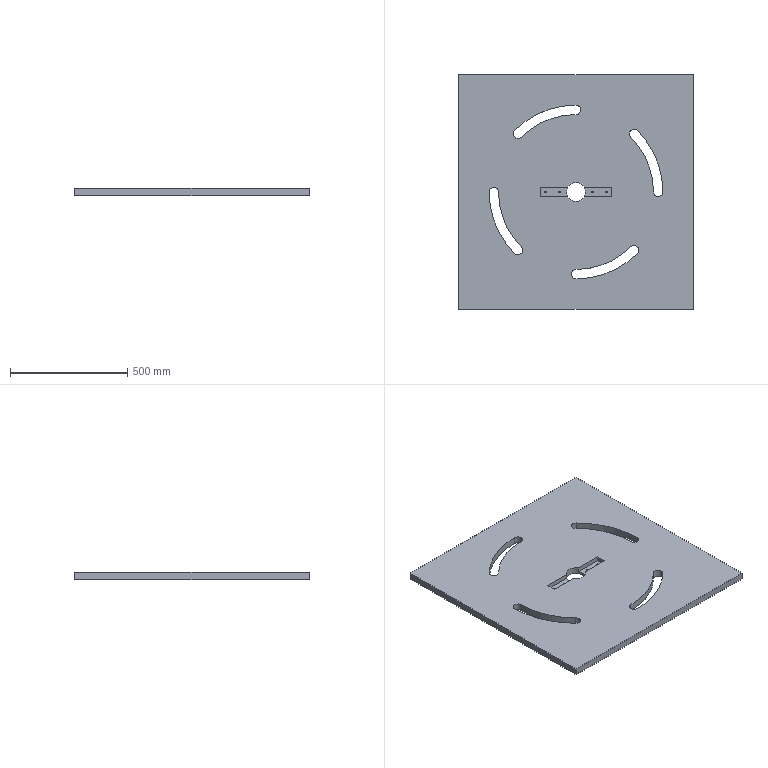Part | SolidWorks | features ICE 3, Extrusion 1, HoleWzd 1 | 1 solid | 43 faces | box 1000 x 1000 x 30 mm | volume 28197892 mm3 | cylinder 29 | plane 14 | commonest cylinder face diameters 40 x11 8.5 x8 660 x4 740 x4 80 x2
STEP:
#1=CARTESIAN_POINT('',(-134.25,0.,0.));
#2=VERTEX_POINT('',#1);
#3=CARTESIAN_POINT('',(-125.75,0.,0.));
#4=VERTEX_POINT('',#3);
#5=CARTESIAN_POINT('',(-130.,0.,0.));
#6=DIRECTION('',(0.,0.,1.));
#7=DIRECTION('',(1.,0.,0.));
#8=AXIS2_PLACEMENT_3D('',#5,#6,#7);
#9=CIRCLE('',#8,4.25);
#10=EDGE_CURVE('',#2,#4,#9,.T.);
#11=ORIENTED_EDGE('',*,*,#10,.F.);
#12=CARTESIAN_POINT('',(-134.25,0.,10.));
#13=VERTEX_POINT('',#12);
#14=CARTESIAN_POINT('',(-134.25,0.,10.));
#15=DIRECTION('',(0.,0.,1.));
#16=VECTOR('',#15,1000.);
#17=LINE('',#14,#16);
#18=EDGE_CURVE('',#2,#13,#17,.T.);
#19=ORIENTED_EDGE('',*,*,#18,.T.);
#20=CARTESIAN_POINT('',(-125.75,0.,10.));
#21=VERTEX_POINT('',#20);
#22=CARTESIAN_POINT('',(-130.,0.,10.));
#23=DIRECTION('',(0.,0.,1.));
#24=DIRECTION('',(1.,0.,0.));
#25=AXIS2_PLACEMENT_3D('',#22,#23,#24);
#26=CIRCLE('',#25,4.25);
#27=EDGE_CURVE('',#13,#21,#26,.T.);
#28=ORIENTED_EDGE('',*,*,#27,.T.);
#29=CARTESIAN_POINT('',(-125.75,0.,10.));
#30=DIRECTION('',(0.,0.,1.));
#31=VECTOR('',#30,1000.);
#32=LINE('',#29,#31);
#33=EDGE_CURVE('',#4,#21,#32,.T.);
#34=ORIENTED_EDGE('',*,*,#33,.F.);
#35=EDGE_LOOP('',(#11,#19,#28,#34));
#36=FACE_OUTER_BOUND('',#35,.T.);
#37=CARTESIAN_POINT('',(-130.,0.,10.));
#38=DIRECTION('',(0.,0.,1.));
#39=DIRECTION('',(1.,0.,0.));
#40=AXIS2_PLACEMENT_3D('',#37,#38,#39);
#41=CYLINDRICAL_SURFACE('',#40,4.25);
#42=ADVANCED_FACE('',(#36),#41,.F.);
#43=CARTESIAN_POINT('',(-74.25,0.,0.));
#44=VERTEX_POINT('',#43);
#45=CARTESIAN_POINT('',(-65.75,0.,0.));
#46=VERTEX_POINT('',#45);
#47=CARTESIAN_POINT('',(-70.,0.,0.));
#48=DIRECTION('',(0.,0.,1.));
#49=DIRECTION('',(1.,0.,0.));
#50=AXIS2_PLACEMENT_3D('',#47,#48,#49);
#51=CIRCLE('',#50,4.25);
#52=EDGE_CURVE('',#44,#46,#51,.T.);
#53=ORIENTED_EDGE('',*,*,#52,.F.);
#54=CARTESIAN_POINT('',(-74.25,0.,10.));
#55=VERTEX_POINT('',#54);
#56=CARTESIAN_POINT('',(-74.25,0.,10.));
#57=DIRECTION('',(0.,0.,1.));
#58=VECTOR('',#57,1000.);
#59=LINE('',#56,#58);
#60=EDGE_CURVE('',#44,#55,#59,.T.);
#61=ORIENTED_EDGE('',*,*,#60,.T.);
#62=CARTESIAN_POINT('',(-65.75,0.,10.));
#63=VERTEX_POINT('',#62);
#64=CARTESIAN_POINT('',(-70.,0.,10.));
#65=DIRECTION('',(0.,0.,1.));
#66=DIRECTION('',(1.,0.,0.));
#67=AXIS2_PLACEMENT_3D('',#64,#65,#66);
#68=CIRCLE('',#67,4.25);
#69=EDGE_CURVE('',#55,#63,#68,.T.);
#70=ORIENTED_EDGE('',*,*,#69,.T.);
#71=CARTESIAN_POINT('',(-65.75,0.,10.));
#72=DIRECTION('',(0.,0.,1.));
#73=VECTOR('',#72,1000.);
#74=LINE('',#71,#73);
#75=EDGE_CURVE('',#46,#63,#74,.T.);
#76=ORIENTED_EDGE('',*,*,#75,.F.);
#77=EDGE_LOOP('',(#53,#61,#70,#76));
#78=FACE_OUTER_BOUND('',#77,.T.);
#79=CARTESIAN_POINT('',(-70.,0.,10.));
#80=DIRECTION('',(0.,0.,1.));
#81=DIRECTION('',(1.,0.,0.));
#82=AXIS2_PLACEMENT_3D('',#79,#80,#81);
#83=CYLINDRICAL_SURFACE('',#82,4.25);
#84=ADVANCED_FACE('',(#78),#83,.F.);
#85=CARTESIAN_POINT('',(65.75,0.,0.));
#86=VERTEX_POINT('',#85);
#87=CARTESIAN_POINT('',(74.25,0.,0.));
#88=VERTEX_POINT('',#87);
#89=CARTESIAN_POINT('',(70.,0.,0.));
#90=DIRECTION('',(0.,0.,1.));
#91=DIRECTION('',(1.,0.,0.));
#92=AXIS2_PLACEMENT_3D('',#89,#90,#91);
#93=CIRCLE('',#92,4.25);
#94=EDGE_CURVE('',#86,#88,#93,.T.);
#95=ORIENTED_EDGE('',*,*,#94,.F.);
#96=CARTESIAN_POINT('',(65.75,0.,10.));
#97=VERTEX_POINT('',#96);
#98=CARTESIAN_POINT('',(65.75,0.,10.));
#99=DIRECTION('',(0.,0.,1.));
#100=VECTOR('',#99,1000.);
#101=LINE('',#98,#100);
#102=EDGE_CURVE('',#86,#97,#101,.T.);
#103=ORIENTED_EDGE('',*,*,#102,.T.);
#104=CARTESIAN_POINT('',(74.25,0.,10.));
#105=VERTEX_POINT('',#104);
#106=CARTESIAN_POINT('',(70.,0.,10.));
#107=DIRECTION('',(0.,0.,1.));
#108=DIRECTION('',(1.,0.,0.));
#109=AXIS2_PLACEMENT_3D('',#106,#107,#108);
#110=CIRCLE('',#109,4.25);
#111=EDGE_CURVE('',#97,#105,#110,.T.);
#112=ORIENTED_EDGE('',*,*,#111,.T.);
#113=CARTESIAN_POINT('',(74.25,0.,10.));
#114=DIRECTION('',(0.,0.,1.));
#115=VECTOR('',#114,1000.);
#116=LINE('',#113,#115);
#117=EDGE_CURVE('',#88,#105,#116,.T.);
#118=ORIENTED_EDGE('',*,*,#117,.F.);
#119=EDGE_LOOP('',(#95,#103,#112,#118));
#120=FACE_OUTER_BOUND('',#119,.T.);
#121=CARTESIAN_POINT('',(70.,0.,10.));
#122=DIRECTION('',(0.,0.,1.));
#123=DIRECTION('',(1.,0.,0.));
#124=AXIS2_PLACEMENT_3D('',#121,#122,#123);
#125=CYLINDRICAL_SURFACE('',#124,4.25);
#126=ADVANCED_FACE('',(#120),#125,.F.);
#127=CARTESIAN_POINT('',(125.75,0.,0.));
#128=VERTEX_POINT('',#127);
#129=CARTESIAN_POINT('',(134.25,0.,0.));
#130=VERTEX_POINT('',#129);
#131=CARTESIAN_POINT('',(130.,0.,0.));
#132=DIRECTION('',(0.,0.,1.));
#133=DIRECTION('',(1.,0.,0.));
#134=AXIS2_PLACEMENT_3D('',#131,#132,#133);
#135=CIRCLE('',#134,4.25);
#136=EDGE_CURVE('',#128,#130,#135,.T.);
#137=ORIENTED_EDGE('',*,*,#136,.F.);
#138=CARTESIAN_POINT('',(125.75,0.,10.));
#139=VERTEX_POINT('',#138);
#140=CARTESIAN_POINT('',(125.75,0.,10.));
#141=DIRECTION('',(0.,0.,1.));
#142=VECTOR('',#141,1000.);
#143=LINE('',#140,#142);
#144=EDGE_CURVE('',#128,#139,#143,.T.);
#145=ORIENTED_EDGE('',*,*,#144,.T.);
#146=CARTESIAN_POINT('',(134.25,0.,10.));
#147=VERTEX_POINT('',#146);
#148=CARTESIAN_POINT('',(130.,0.,10.));
#149=DIRECTION('',(0.,0.,1.));
#150=DIRECTION('',(1.,0.,0.));
#151=AXIS2_PLACEMENT_3D('',#148,#149,#150);
#152=CIRCLE('',#151,4.25);
#153=EDGE_CURVE('',#139,#147,#152,.T.);
#154=ORIENTED_EDGE('',*,*,#153,.T.);
#155=CARTESIAN_POINT('',(134.25,0.,10.));
#156=DIRECTION('',(0.,0.,1.));
#157=VECTOR('',#156,1000.);
#158=LINE('',#155,#157);
#159=EDGE_CURVE('',#130,#147,#158,.T.);
#160=ORIENTED_EDGE('',*,*,#159,.F.);
#161=EDGE_LOOP('',(#137,#145,#154,#160));
#162=FACE_OUTER_BOUND('',#161,.T.);
#163=CARTESIAN_POINT('',(130.,0.,10.));
#164=DIRECTION('',(0.,0.,1.));
#165=DIRECTION('',(1.,0.,0.));
#166=AXIS2_PLACEMENT_3D('',#163,#164,#165);
#167=CYLINDRICAL_SURFACE('',#166,4.25);
#168=ADVANCED_FACE('',(#162),#167,.F.);
#169=CARTESIAN_POINT('',(-40.,0.,0.));
#170=VERTEX_POINT('',#169);
#171=CARTESIAN_POINT('',(40.,0.,0.));
#172=VERTEX_POINT('',#171);
#173=CARTESIAN_POINT('',(0.,0.,0.));
#174=DIRECTION('',(0.,0.,1.));
#175=DIRECTION('',(1.,0.,0.));
#176=AXIS2_PLACEMENT_3D('',#173,#174,#175);
#177=CIRCLE('',#176,40.);
#178=EDGE_CURVE('',#170,#172,#177,.T.);
#179=ORIENTED_EDGE('',*,*,#178,.F.);
#180=CARTESIAN_POINT('',(-40.,0.,10.));
#181=VERTEX_POINT('',#180);
#182=CARTESIAN_POINT('',(-40.,0.,0.));
#183=DIRECTION('',(0.,0.,1.));
#184=VECTOR('',#183,1000.);
#185=LINE('',#182,#184);
#186=EDGE_CURVE('',#170,#181,#185,.T.);
#187=ORIENTED_EDGE('',*,*,#186,.T.);
#188=CARTESIAN_POINT('',(-34.641,-20.,10.));
#189=VERTEX_POINT('',#188);
#190=CARTESIAN_POINT('',(0.,0.,10.));
#191=DIRECTION('',(0.,0.,1.));
#192=DIRECTION('',(-1.,0.,0.));
#193=AXIS2_PLACEMENT_3D('',#190,#191,#192);
#194=CIRCLE('',#193,40.);
#195=EDGE_CURVE('',#181,#189,#194,.T.);
#196=ORIENTED_EDGE('',*,*,#195,.T.);
#197=CARTESIAN_POINT('',(-34.641,-20.,30.));
#198=VERTEX_POINT('',#197);
#199=CARTESIAN_POINT('',(-34.641,-20.,0.));
#200=DIRECTION('',(0.,0.,1.));
#201=VECTOR('',#200,1000.);
#202=LINE('',#199,#201);
#203=EDGE_CURVE('',#189,#198,#202,.T.);
#204=ORIENTED_EDGE('',*,*,#203,.T.);
#205=CARTESIAN_POINT('',(34.641,-20.,30.));
#206=VERTEX_POINT('',#205);
#207=CARTESIAN_POINT('',(0.,0.,30.));
#208=DIRECTION('',(0.,0.,1.));
#209=DIRECTION('',(1.,0.,0.));
#210=AXIS2_PLACEMENT_3D('',#207,#208,#209);
#211=CIRCLE('',#210,40.);
#212=EDGE_CURVE('',#198,#206,#211,.T.);
#213=ORIENTED_EDGE('',*,*,#212,.T.);
#214=CARTESIAN_POINT('',(34.641,-20.,10.));
#215=VERTEX_POINT('',#214);
#216=CARTESIAN_POINT('',(34.641,-20.,0.));
#217=DIRECTION('',(0.,0.,-1.));
#218=VECTOR('',#217,1000.);
#219=LINE('',#216,#218);
#220=EDGE_CURVE('',#206,#215,#219,.T.);
#221=ORIENTED_EDGE('',*,*,#220,.T.);
#222=CARTESIAN_POINT('',(40.,0.,10.));
#223=VERTEX_POINT('',#222);
#224=CARTESIAN_POINT('',(0.,0.,10.));
#225=DIRECTION('',(0.,0.,1.));
#226=DIRECTION('',(-1.,0.,0.));
#227=AXIS2_PLACEMENT_3D('',#224,#225,#226);
#228=CIRCLE('',#227,40.);
#229=EDGE_CURVE('',#215,#223,#228,.T.);
#230=ORIENTED_EDGE('',*,*,#229,.T.);
#231=CARTESIAN_POINT('',(40.,0.,0.));
#232=DIRECTION('',(0.,0.,1.));
#233=VECTOR('',#232,1000.);
#234=LINE('',#231,#233);
#235=EDGE_CURVE('',#172,#223,#234,.T.);
#236=ORIENTED_EDGE('',*,*,#235,.F.);
#237=EDGE_LOOP('',(#179,#187,#196,#204,#213,#221,#230,#236));
#238=FACE_OUTER_BOUND('',#237,.T.);
#239=CARTESIAN_POINT('',(0.,0.,0.));
#240=DIRECTION('',(0.,0.,1.));
#241=DIRECTION('',(1.,0.,0.));
#242=AXIS2_PLACEMENT_3D('',#239,#240,#241);
#243=CYLINDRICAL_SURFACE('',#242,40.);
#244=ADVANCED_FACE('',(#238),#243,.F.);
#245=CARTESIAN_POINT('',(-227.487,-247.487,0.));
#246=VERTEX_POINT('',#245);
#247=CARTESIAN_POINT('',(-233.345,-233.345,0.));
#248=VERTEX_POINT('',#247);
#249=CARTESIAN_POINT('',(-247.487,-247.487,0.));
#250=DIRECTION('',(0.,0.,1.));
#251=DIRECTION('',(1.,0.,0.));
#252=AXIS2_PLACEMENT_3D('',#249,#250,#251);
#253=CIRCLE('',#252,20.);
#254=EDGE_CURVE('',#246,#248,#253,.T.);
#255=ORIENTED_EDGE('',*,*,#254,.F.);
#256=CARTESIAN_POINT('',(-227.487,-247.487,30.));
#257=VERTEX_POINT('',#256);
#258=CARTESIAN_POINT('',(-227.487,-247.487,0.));
#259=DIRECTION('',(0.,0.,1.));
#260=VECTOR('',#259,1000.);
#261=LINE('',#258,#260);
#262=EDGE_CURVE('',#246,#257,#261,.T.);
#263=ORIENTED_EDGE('',*,*,#262,.T.);
#264=CARTESIAN_POINT('',(-233.345,-233.345,30.));
#265=VERTEX_POINT('',#264);
#266=CARTESIAN_POINT('',(-247.487,-247.487,30.));
#267=DIRECTION('',(0.,0.,1.));
#268=DIRECTION('',(1.,0.,0.));
#269=AXIS2_PLACEMENT_3D('',#266,#267,#268);
#270=CIRCLE('',#269,20.);
#271=EDGE_CURVE('',#257,#265,#270,.T.);
#272=ORIENTED_EDGE('',*,*,#271,.T.);
#273=CARTESIAN_POINT('',(-233.345,-233.345,0.));
#274=DIRECTION('',(0.,0.,1.));
#275=VECTOR('',#274,1000.);
#276=LINE('',#273,#275);
#277=EDGE_CURVE('',#248,#265,#276,.T.);
#278=ORIENTED_EDGE('',*,*,#277,.F.);
#279=EDGE_LOOP('',(#255,#263,#272,#278));
#280=FACE_OUTER_BOUND('',#279,.T.);
#281=CARTESIAN_POINT('',(-247.487,-247.487,0.));
#282=DIRECTION('',(0.,0.,1.));
#283=DIRECTION('',(1.,0.,0.));
#284=AXIS2_PLACEMENT_3D('',#281,#282,#283);
#285=CYLINDRICAL_SURFACE('',#284,20.);
#286=ADVANCED_FACE('',(#280),#285,.F.);
#287=CARTESIAN_POINT('',(267.487,-247.487,0.));
#288=VERTEX_POINT('',#287);
#289=CARTESIAN_POINT('',(233.345,-233.345,0.));
#290=VERTEX_POINT('',#289);
#291=CARTESIAN_POINT('',(247.487,-247.487,0.));
#292=DIRECTION('',(0.,0.,1.));
#293=DIRECTION('',(1.,0.,0.));
#294=AXIS2_PLACEMENT_3D('',#291,#292,#293);
#295=CIRCLE('',#294,20.);
#296=EDGE_CURVE('',#288,#290,#295,.T.);
#297=ORIENTED_EDGE('',*,*,#296,.F.);
#298=CARTESIAN_POINT('',(267.487,-247.487,30.));
#299=VERTEX_POINT('',#298);
#300=CARTESIAN_POINT('',(267.487,-247.487,0.));
#301=DIRECTION('',(0.,0.,1.));
#302=VECTOR('',#301,1000.);
#303=LINE('',#300,#302);
#304=EDGE_CURVE('',#288,#299,#303,.T.);
#305=ORIENTED_EDGE('',*,*,#304,.T.);
#306=CARTESIAN_POINT('',(233.345,-233.345,30.));
#307=VERTEX_POINT('',#306);
#308=CARTESIAN_POINT('',(247.487,-247.487,30.));
#309=DIRECTION('',(0.,0.,1.));
#310=DIRECTION('',(1.,0.,0.));
#311=AXIS2_PLACEMENT_3D('',#308,#309,#310);
#312=CIRCLE('',#311,20.);
#313=EDGE_CURVE('',#299,#307,#312,.T.);
#314=ORIENTED_EDGE('',*,*,#313,.T.);
#315=CARTESIAN_POINT('',(233.345,-233.345,0.));
#316=DIRECTION('',(0.,0.,1.));
#317=VECTOR('',#316,1000.);
#318=LINE('',#315,#317);
#319=EDGE_CURVE('',#290,#307,#318,.T.);
#320=ORIENTED_EDGE('',*,*,#319,.F.);
#321=EDGE_LOOP('',(#297,#305,#314,#320));
#322=FACE_OUTER_BOUND('',#321,.T.);
#323=CARTESIAN_POINT('',(247.487,-247.487,0.));
#324=DIRECTION('',(0.,0.,1.));
#325=DIRECTION('',(1.,0.,0.));
#326=AXIS2_PLACEMENT_3D('',#323,#324,#325);
#327=CYLINDRICAL_SURFACE('',#326,20.);
#328=ADVANCED_FACE('',(#322),#327,.F.);
#329=CARTESIAN_POINT('',(20.,350.,0.));
#330=VERTEX_POINT('',#329);
#331=CARTESIAN_POINT('',(0.,370.,0.));
#332=VERTEX_POINT('',#331);
#333=CARTESIAN_POINT('',(0.,350.,0.));
#334=DIRECTION('',(0.,0.,1.));
#335=DIRECTION('',(1.,0.,0.));
#336=AXIS2_PLACEMENT_3D('',#333,#334,#335);
#337=CIRCLE('',#336,20.);
#338=EDGE_CURVE('',#330,#332,#337,.T.);
#339=ORIENTED_EDGE('',*,*,#338,.F.);
#340=CARTESIAN_POINT('',(20.,350.,30.));
#341=VERTEX_POINT('',#340);
#342=CARTESIAN_POINT('',(20.,350.,0.));
#343=DIRECTION('',(0.,0.,1.));
#344=VECTOR('',#343,1000.);
#345=LINE('',#342,#344);
#346=EDGE_CURVE('',#330,#341,#345,.T.);
#347=ORIENTED_EDGE('',*,*,#346,.T.);
#348=CARTESIAN_POINT('',(0.,370.,30.));
#349=VERTEX_POINT('',#348);
#350=CARTESIAN_POINT('',(0.,350.,30.));
#351=DIRECTION('',(0.,0.,1.));
#352=DIRECTION('',(1.,0.,0.));
#353=AXIS2_PLACEMENT_3D('',#350,#351,#352);
#354=CIRCLE('',#353,20.);
#355=EDGE_CURVE('',#341,#349,#354,.T.);
#356=ORIENTED_EDGE('',*,*,#355,.T.);
#357=CARTESIAN_POINT('',(0.,370.,0.));
#358=DIRECTION('',(0.,0.,1.));
#359=VECTOR('',#358,1000.);
#360=LINE('',#357,#359);
#361=EDGE_CURVE('',#332,#349,#360,.T.);
#362=ORIENTED_EDGE('',*,*,#361,.F.);
#363=EDGE_LOOP('',(#339,#347,#356,#362));
#364=FACE_OUTER_BOUND('',#363,.T.);
#365=CARTESIAN_POINT('',(0.,350.,0.));
#366=DIRECTION('',(0.,0.,1.));
#367=DIRECTION('',(1.,0.,0.));
#368=AXIS2_PLACEMENT_3D('',#365,#366,#367);
#369=CYLINDRICAL_SURFACE('',#368,20.);
#370=ADVANCED_FACE('',(#364),#369,.F.);
#371=CARTESIAN_POINT('',(130.,0.,0.));
#372=DIRECTION('',(0.,0.,1.));
#373=DIRECTION('',(1.,0.,0.));
#374=AXIS2_PLACEMENT_3D('',#371,#372,#373);
#375=CIRCLE('',#374,4.25);
#376=EDGE_CURVE('',#130,#128,#375,.T.);
#377=ORIENTED_EDGE('',*,*,#376,.T.);
#378=ORIENTED_EDGE('',*,*,#136,.T.);
#379=EDGE_LOOP('',(#377,#378));
#380=FACE_BOUND('',#379,.T.);
#381=CARTESIAN_POINT('',(0.,0.,0.));
#382=DIRECTION('',(0.,0.,1.));
#383=DIRECTION('',(1.,0.,0.));
#384=AXIS2_PLACEMENT_3D('',#381,#382,#383);
#385=CIRCLE('',#384,40.);
#386=EDGE_CURVE('',#172,#170,#385,.T.);
#387=ORIENTED_EDGE('',*,*,#386,.T.);
#388=ORIENTED_EDGE('',*,*,#178,.T.);
#389=EDGE_LOOP('',(#387,#388));
#390=FACE_BOUND('',#389,.T.);
#391=CARTESIAN_POINT('',(-330.,0.,0.));
#392=VERTEX_POINT('',#391);
#393=CARTESIAN_POINT('',(-370.,0.,0.));
#394=VERTEX_POINT('',#393);
#395=CARTESIAN_POINT('',(-350.,0.,0.));
#396=DIRECTION('',(0.,0.,1.));
#397=DIRECTION('',(1.,0.,0.));
#398=AXIS2_PLACEMENT_3D('',#395,#396,#397);
#399=CIRCLE('',#398,20.);
#400=EDGE_CURVE('',#392,#394,#399,.T.);
#401=ORIENTED_EDGE('',*,*,#400,.T.);
#402=CARTESIAN_POINT('',(-261.63,-261.63,0.));
#403=VERTEX_POINT('',#402);
#404=CARTESIAN_POINT('',(0.,0.,0.));
#405=DIRECTION('',(0.,0.,1.));
#406=DIRECTION('',(1.,0.,0.));
#407=AXIS2_PLACEMENT_3D('',#404,#405,#406);
#408=CIRCLE('',#407,370.);
#409=EDGE_CURVE('',#394,#403,#408,.T.);
#410=ORIENTED_EDGE('',*,*,#409,.T.);
#411=CARTESIAN_POINT('',(-247.487,-247.487,0.));
#412=DIRECTION('',(0.,0.,1.));
#413=DIRECTION('',(1.,0.,0.));
#414=AXIS2_PLACEMENT_3D('',#411,#412,#413);
#415=CIRCLE('',#414,20.);
#416=EDGE_CURVE('',#403,#246,#415,.T.);
#417=ORIENTED_EDGE('',*,*,#416,.T.);
#418=ORIENTED_EDGE('',*,*,#254,.T.);
#419=CARTESIAN_POINT('',(0.,0.,0.));
#420=DIRECTION('',(0.,0.,-1.));
#421=DIRECTION('',(1.,0.,0.));
#422=AXIS2_PLACEMENT_3D('',#419,#420,#421);
#423=CIRCLE('',#422,330.);
#424=EDGE_CURVE('',#248,#392,#423,.T.);
#425=ORIENTED_EDGE('',*,*,#424,.T.);
#426=EDGE_LOOP('',(#401,#410,#417,#418,#425));
#427=FACE_BOUND('',#426,.T.);
#428=CARTESIAN_POINT('',(0.,-330.,0.));
#429=VERTEX_POINT('',#428);
#430=CARTESIAN_POINT('',(0.,-370.,0.));
#431=VERTEX_POINT('',#430);
#432=CARTESIAN_POINT('',(0.,-350.,0.));
#433=DIRECTION('',(0.,0.,1.));
#434=DIRECTION('',(1.,0.,0.));
#435=AXIS2_PLACEMENT_3D('',#432,#433,#434);
#436=CIRCLE('',#435,20.);
#437=EDGE_CURVE('',#429,#431,#436,.T.);
#438=ORIENTED_EDGE('',*,*,#437,.T.);
#439=CARTESIAN_POINT('',(261.63,-261.63,0.));
#440=VERTEX_POINT('',#439);
#441=CARTESIAN_POINT('',(0.,0.,0.));
#442=DIRECTION('',(0.,0.,1.));
#443=DIRECTION('',(1.,0.,0.));
#444=AXIS2_PLACEMENT_3D('',#441,#442,#443);
#445=CIRCLE('',#444,370.);
#446=EDGE_CURVE('',#431,#440,#445,.T.);
#447=ORIENTED_EDGE('',*,*,#446,.T.);
#448=CARTESIAN_POINT('',(247.487,-247.487,0.));
#449=DIRECTION('',(0.,0.,1.));
#450=DIRECTION('',(1.,0.,0.));
#451=AXIS2_PLACEMENT_3D('',#448,#449,#450);
#452=CIRCLE('',#451,20.);
#453=EDGE_CURVE('',#440,#288,#452,.T.);
#454=ORIENTED_EDGE('',*,*,#453,.T.);
#455=ORIENTED_EDGE('',*,*,#296,.T.);
#456=CARTESIAN_POINT('',(0.,0.,0.));
#457=DIRECTION('',(0.,0.,-1.));
#458=DIRECTION('',(1.,0.,0.));
#459=AXIS2_PLACEMENT_3D('',#456,#457,#458);
#460=CIRCLE('',#459,330.);
#461=EDGE_CURVE('',#290,#429,#460,.T.);
#462=ORIENTED_EDGE('',*,*,#461,.T.);
#463=EDGE_LOOP('',(#438,#447,#454,#455,#462));
#464=FACE_BOUND('',#463,.T.);
#465=CARTESIAN_POINT('',(330.,0.,0.));
#466=VERTEX_POINT('',#465);
#467=CARTESIAN_POINT('',(370.,0.,0.));
#468=VERTEX_POINT('',#467);
#469=CARTESIAN_POINT('',(350.,0.,0.));
#470=DIRECTION('',(0.,0.,1.));
#471=DIRECTION('',(1.,0.,0.));
#472=AXIS2_PLACEMENT_3D('',#469,#470,#471);
#473=CIRCLE('',#472,20.);
#474=EDGE_CURVE('',#466,#468,#473,.T.);
#475=ORIENTED_EDGE('',*,*,#474,.T.);
#476=CARTESIAN_POINT('',(261.63,261.63,0.));
#477=VERTEX_POINT('',#476);
#478=CARTESIAN_POINT('',(0.,0.,0.));
#479=DIRECTION('',(0.,0.,1.));
#480=DIRECTION('',(1.,0.,0.));
#481=AXIS2_PLACEMENT_3D('',#478,#479,#480);
#482=CIRCLE('',#481,370.);
#483=EDGE_CURVE('',#468,#477,#482,.T.);
#484=ORIENTED_EDGE('',*,*,#483,.T.);
#485=CARTESIAN_POINT('',(233.345,233.345,0.));
#486=VERTEX_POINT('',#485);
#487=CARTESIAN_POINT('',(247.487,247.487,0.));
#488=DIRECTION('',(0.,0.,1.));
#489=DIRECTION('',(1.,0.,0.));
#490=AXIS2_PLACEMENT_3D('',#487,#488,#489);
#491=CIRCLE('',#490,20.);
#492=EDGE_CURVE('',#477,#486,#491,.T.);
#493=ORIENTED_EDGE('',*,*,#492,.T.);
#494=CARTESIAN_POINT('',(0.,0.,0.));
#495=DIRECTION('',(0.,0.,-1.));
#496=DIRECTION('',(1.,0.,0.));
#497=AXIS2_PLACEMENT_3D('',#494,#495,#496);
#498=CIRCLE('',#497,330.);
#499=EDGE_CURVE('',#486,#466,#498,.T.);
#500=ORIENTED_EDGE('',*,*,#499,.T.);
#501=EDGE_LOOP('',(#475,#484,#493,#500));
#502=FACE_BOUND('',#501,.T.);
#503=CARTESIAN_POINT('',(0.,330.,0.));
#504=VERTEX_POINT('',#503);
#505=CARTESIAN_POINT('',(0.,350.,0.));
#506=DIRECTION('',(0.,0.,1.));
#507=DIRECTION('',(1.,0.,0.));
#508=AXIS2_PLACEMENT_3D('',#505,#506,#507);
#509=CIRCLE('',#508,20.);
#510=EDGE_CURVE('',#504,#330,#509,.T.);
#511=ORIENTED_EDGE('',*,*,#510,.T.);
#512=ORIENTED_EDGE('',*,*,#338,.T.);
#513=CARTESIAN_POINT('',(-261.63,261.63,0.));
#514=VERTEX_POINT('',#513);
#515=CARTESIAN_POINT('',(0.,0.,0.));
#516=DIRECTION('',(0.,0.,1.));
#517=DIRECTION('',(1.,0.,0.));
#518=AXIS2_PLACEMENT_3D('',#515,#516,#517);
#519=CIRCLE('',#518,370.);
#520=EDGE_CURVE('',#332,#514,#519,.T.);
#521=ORIENTED_EDGE('',*,*,#520,.T.);
#522=CARTESIAN_POINT('',(-233.345,233.345,0.));
#523=VERTEX_POINT('',#522);
#524=CARTESIAN_POINT('',(-247.487,247.487,0.));
#525=DIRECTION('',(0.,0.,1.));
#526=DIRECTION('',(1.,0.,0.));
#527=AXIS2_PLACEMENT_3D('',#524,#525,#526);
#528=CIRCLE('',#527,20.);
#529=EDGE_CURVE('',#514,#523,#528,.T.);
#530=ORIENTED_EDGE('',*,*,#529,.T.);
#531=CARTESIAN_POINT('',(0.,0.,0.));
#532=DIRECTION('',(0.,0.,-1.));
#533=DIRECTION('',(1.,0.,0.));
#534=AXIS2_PLACEMENT_3D('',#531,#532,#533);
#535=CIRCLE('',#534,330.);
#536=EDGE_CURVE('',#523,#504,#535,.T.);
#537=ORIENTED_EDGE('',*,*,#536,.T.);
#538=EDGE_LOOP('',(#511,#512,#521,#530,#537));
#539=FACE_BOUND('',#538,.T.);
#540=CARTESIAN_POINT('',(500.,-500.,0.));
#541=VERTEX_POINT('',#540);
#542=CARTESIAN_POINT('',(500.,500.,0.));
#543=VERTEX_POINT('',#542);
#544=CARTESIAN_POINT('',(500.,-500.,0.));
#545=DIRECTION('',(0.,1.,0.));
#546=VECTOR('',#545,1000.);
#547=LINE('',#544,#546);
#548=EDGE_CURVE('',#541,#543,#547,.T.);
#549=ORIENTED_EDGE('',*,*,#548,.F.);
#550=CARTESIAN_POINT('',(-500.,-500.,0.));
#551=VERTEX_POINT('',#550);
#552=CARTESIAN_POINT('',(-500.,-500.,0.));
#553=DIRECTION('',(1.,0.,0.));
#554=VECTOR('',#553,1000.);
#555=LINE('',#552,#554);
#556=EDGE_CURVE('',#551,#541,#555,.T.);
#557=ORIENTED_EDGE('',*,*,#556,.F.);
#558=CARTESIAN_POINT('',(-500.,500.,0.));
#559=VERTEX_POINT('',#558);
#560=CARTESIAN_POINT('',(-500.,-500.,0.));
#561=DIRECTION('',(0.,-1.,0.));
#562=VECTOR('',#561,1000.);
#563=LINE('',#560,#562);
#564=EDGE_CURVE('',#559,#551,#563,.T.);
#565=ORIENTED_EDGE('',*,*,#564,.F.);
#566=CARTESIAN_POINT('',(-500.,500.,0.));
#567=DIRECTION('',(-1.,0.,0.));
#568=VECTOR('',#567,1000.);
#569=LINE('',#566,#568);
#570=EDGE_CURVE('',#543,#559,#569,.T.);
#571=ORIENTED_EDGE('',*,*,#570,.F.);
#572=EDGE_LOOP('',(#549,#557,#565,#571));
#573=FACE_OUTER_BOUND('',#572,.T.);
#574=CARTESIAN_POINT('',(70.,0.,0.));
#575=DIRECTION('',(0.,0.,1.));
#576=DIRECTION('',(1.,0.,0.));
#577=AXIS2_PLACEMENT_3D('',#574,#575,#576);
#578=CIRCLE('',#577,4.25);
#579=EDGE_CURVE('',#88,#86,#578,.T.);
#580=ORIENTED_EDGE('',*,*,#579,.T.);
#581=ORIENTED_EDGE('',*,*,#94,.T.);
#582=EDGE_LOOP('',(#580,#581));
#583=FACE_BOUND('',#582,.T.);
#584=CARTESIAN_POINT('',(-70.,0.,0.));
#585=DIRECTION('',(0.,0.,1.));
#586=DIRECTION('',(1.,0.,0.));
#587=AXIS2_PLACEMENT_3D('',#584,#585,#586);
#588=CIRCLE('',#587,4.25);
#589=EDGE_CURVE('',#46,#44,#588,.T.);
#590=ORIENTED_EDGE('',*,*,#589,.T.);
#591=ORIENTED_EDGE('',*,*,#52,.T.);
#592=EDGE_LOOP('',(#590,#591));
#593=FACE_BOUND('',#592,.T.);
#594=CARTESIAN_POINT('',(-130.,0.,0.));
#595=DIRECTION('',(0.,0.,1.));
#596=DIRECTION('',(1.,0.,0.));
#597=AXIS2_PLACEMENT_3D('',#594,#595,#596);
#598=CIRCLE('',#597,4.25);
#599=EDGE_CURVE('',#4,#2,#598,.T.);
#600=ORIENTED_EDGE('',*,*,#599,.T.);
#601=ORIENTED_EDGE('',*,*,#10,.T.);
#602=EDGE_LOOP('',(#600,#601));
#603=FACE_BOUND('',#602,.T.);
#604=CARTESIAN_POINT('',(0.,0.,0.));
#605=DIRECTION('',(0.,0.,-1.));
#606=DIRECTION('',(-1.,0.,0.));
#607=AXIS2_PLACEMENT_3D('',#604,#605,#606);
#608=PLANE('',#607);
#609=ADVANCED_FACE('',(#380,#390,#427,#464,#502,#539,#573,#583,#593,#603),#608,.T.);
#610=ORIENTED_EDGE('',*,*,#548,.T.);
#611=CARTESIAN_POINT('',(500.,500.,30.));
#612=VERTEX_POINT('',#611);
#613=CARTESIAN_POINT('',(500.,500.,30.));
#614=DIRECTION('',(0.,0.,-1.));
#615=VECTOR('',#614,1000.);
#616=LINE('',#613,#615);
#617=EDGE_CURVE('',#612,#543,#616,.T.);
#618=ORIENTED_EDGE('',*,*,#617,.F.);
#619=CARTESIAN_POINT('',(500.,-500.,30.));
#620=VERTEX_POINT('',#619);
#621=CARTESIAN_POINT('',(500.,-500.,30.));
#622=DIRECTION('',(0.,1.,0.));
#623=VECTOR('',#622,1000.);
#624=LINE('',#621,#623);
#625=EDGE_CURVE('',#620,#612,#624,.T.);
#626=ORIENTED_EDGE('',*,*,#625,.F.);
#627=CARTESIAN_POINT('',(500.,-500.,30.));
#628=DIRECTION('',(0.,0.,-1.));
#629=VECTOR('',#628,1000.);
#630=LINE('',#627,#629);
#631=EDGE_CURVE('',#620,#541,#630,.T.);
#632=ORIENTED_EDGE('',*,*,#631,.T.);
#633=EDGE_LOOP('',(#610,#618,#626,#632));
#634=FACE_OUTER_BOUND('',#633,.T.);
#635=CARTESIAN_POINT('',(500.,-500.,30.));
#636=DIRECTION('',(-1.,0.,0.));
#637=DIRECTION('',(0.,0.,1.));
#638=AXIS2_PLACEMENT_3D('',#635,#636,#637);
#639=PLANE('',#638);
#640=ADVANCED_FACE('',(#634),#639,.F.);
#641=ORIENTED_EDGE('',*,*,#570,.T.);
#642=CARTESIAN_POINT('',(-500.,500.,30.));
#643=VERTEX_POINT('',#642);
#644=CARTESIAN_POINT('',(-500.,500.,30.));
#645=DIRECTION('',(0.,0.,-1.));
#646=VECTOR('',#645,1000.);
#647=LINE('',#644,#646);
#648=EDGE_CURVE('',#643,#559,#647,.T.);
#649=ORIENTED_EDGE('',*,*,#648,.F.);
#650=CARTESIAN_POINT('',(-500.,500.,30.));
#651=DIRECTION('',(-1.,0.,0.));
#652=VECTOR('',#651,1000.);
#653=LINE('',#650,#652);
#654=EDGE_CURVE('',#612,#643,#653,.T.);
#655=ORIENTED_EDGE('',*,*,#654,.F.);
#656=ORIENTED_EDGE('',*,*,#617,.T.);
#657=EDGE_LOOP('',(#641,#649,#655,#656));
#658=FACE_OUTER_BOUND('',#657,.T.);
#659=CARTESIAN_POINT('',(-500.,500.,30.));
#660=DIRECTION('',(0.,-1.,0.));
#661=DIRECTION('',(0.,0.,-1.));
#662=AXIS2_PLACEMENT_3D('',#659,#660,#661);
#663=PLANE('',#662);
#664=ADVANCED_FACE('',(#658),#663,.F.);
#665=ORIENTED_EDGE('',*,*,#564,.T.);
#666=CARTESIAN_POINT('',(-500.,-500.,30.));
#667=VERTEX_POINT('',#666);
#668=CARTESIAN_POINT('',(-500.,-500.,30.));
#669=DIRECTION('',(0.,0.,-1.));
#670=VECTOR('',#669,1000.);
#671=LINE('',#668,#670);
#672=EDGE_CURVE('',#667,#551,#671,.T.);
#673=ORIENTED_EDGE('',*,*,#672,.F.);
#674=CARTESIAN_POINT('',(-500.,-500.,30.));
#675=DIRECTION('',(0.,-1.,0.));
#676=VECTOR('',#675,1000.);
#677=LINE('',#674,#676);
#678=EDGE_CURVE('',#643,#667,#677,.T.);
#679=ORIENTED_EDGE('',*,*,#678,.F.);
#680=ORIENTED_EDGE('',*,*,#648,.T.);
#681=EDGE_LOOP('',(#665,#673,#679,#680));
#682=FACE_OUTER_BOUND('',#681,.T.);
#683=CARTESIAN_POINT('',(-500.,-500.,30.));
#684=DIRECTION('',(1.,0.,0.));
#685=DIRECTION('',(0.,0.,-1.));
#686=AXIS2_PLACEMENT_3D('',#683,#684,#685);
#687=PLANE('',#686);
#688=ADVANCED_FACE('',(#682),#687,.F.);
#689=ORIENTED_EDGE('',*,*,#556,.T.);
#690=ORIENTED_EDGE('',*,*,#631,.F.);
#691=CARTESIAN_POINT('',(-500.,-500.,30.));
#692=DIRECTION('',(1.,0.,0.));
#693=VECTOR('',#692,1000.);
#694=LINE('',#691,#693);
#695=EDGE_CURVE('',#667,#620,#694,.T.);
#696=ORIENTED_EDGE('',*,*,#695,.F.);
#697=ORIENTED_EDGE('',*,*,#672,.T.);
#698=EDGE_LOOP('',(#689,#690,#696,#697));
#699=FACE_OUTER_BOUND('',#698,.T.);
#700=CARTESIAN_POINT('',(-500.,-500.,30.));
#701=DIRECTION('',(0.,1.,0.));
#702=DIRECTION('',(0.,0.,1.));
#703=AXIS2_PLACEMENT_3D('',#700,#701,#702);
#704=PLANE('',#703);
#705=ADVANCED_FACE('',(#699),#704,.F.);
#706=ORIENTED_EDGE('',*,*,#212,.F.);
#707=CARTESIAN_POINT('',(-150.,-20.,30.));
#708=VERTEX_POINT('',#707);
#709=CARTESIAN_POINT('',(-150.,-20.,30.));
#710=DIRECTION('',(1.,0.,0.));
#711=VECTOR('',#710,1000.);
#712=LINE('',#709,#711);
#713=EDGE_CURVE('',#708,#198,#712,.T.);
#714=ORIENTED_EDGE('',*,*,#713,.F.);
#715=CARTESIAN_POINT('',(-150.,20.,30.));
#716=VERTEX_POINT('',#715);
#717=CARTESIAN_POINT('',(-150.,-20.,30.));
#718=DIRECTION('',(0.,-1.,0.));
#719=VECTOR('',#718,1000.);
#720=LINE('',#717,#719);
#721=EDGE_CURVE('',#716,#708,#720,.T.);
#722=ORIENTED_EDGE('',*,*,#721,.F.);
#723=CARTESIAN_POINT('',(-34.641,20.,30.));
#724=VERTEX_POINT('',#723);
#725=CARTESIAN_POINT('',(-150.,20.,30.));
#726=DIRECTION('',(-1.,0.,0.));
#727=VECTOR('',#726,1000.);
#728=LINE('',#725,#727);
#729=EDGE_CURVE('',#724,#716,#728,.T.);
#730=ORIENTED_EDGE('',*,*,#729,.F.);
#731=CARTESIAN_POINT('',(34.641,20.,30.));
#732=VERTEX_POINT('',#731);
#733=CARTESIAN_POINT('',(0.,0.,30.));
#734=DIRECTION('',(0.,0.,1.));
#735=DIRECTION('',(1.,0.,0.));
#736=AXIS2_PLACEMENT_3D('',#733,#734,#735);
#737=CIRCLE('',#736,40.);
#738=EDGE_CURVE('',#732,#724,#737,.T.);
#739=ORIENTED_EDGE('',*,*,#738,.F.);
#740=CARTESIAN_POINT('',(150.,20.,30.));
#741=VERTEX_POINT('',#740);
#742=CARTESIAN_POINT('',(150.,20.,30.));
#743=DIRECTION('',(-1.,0.,0.));
#744=VECTOR('',#743,1000.);
#745=LINE('',#742,#744);
#746=EDGE_CURVE('',#741,#732,#745,.T.);
#747=ORIENTED_EDGE('',*,*,#746,.F.);
#748=CARTESIAN_POINT('',(150.,-20.,30.));
#749=VERTEX_POINT('',#748);
#750=CARTESIAN_POINT('',(150.,-20.,30.));
#751=DIRECTION('',(0.,1.,0.));
#752=VECTOR('',#751,1000.);
#753=LINE('',#750,#752);
#754=EDGE_CURVE('',#749,#741,#753,.T.);
#755=ORIENTED_EDGE('',*,*,#754,.F.);
#756=CARTESIAN_POINT('',(150.,-20.,30.));
#757=DIRECTION('',(1.,0.,0.));
#758=VECTOR('',#757,1000.);
#759=LINE('',#756,#758);
#760=EDGE_CURVE('',#206,#749,#759,.T.);
#761=ORIENTED_EDGE('',*,*,#760,.F.);
#762=EDGE_LOOP('',(#706,#714,#722,#730,#739,#747,#755,#761));
#763=FACE_BOUND('',#762,.T.);
#764=CARTESIAN_POINT('',(-370.,0.,30.));
#765=VERTEX_POINT('',#764);
#766=CARTESIAN_POINT('',(-261.63,-261.63,30.));
#767=VERTEX_POINT('',#766);
#768=CARTESIAN_POINT('',(0.,0.,30.));
#769=DIRECTION('',(0.,0.,1.));
#770=DIRECTION('',(1.,0.,0.));
#771=AXIS2_PLACEMENT_3D('',#768,#769,#770);
#772=CIRCLE('',#771,370.);
#773=EDGE_CURVE('',#765,#767,#772,.T.);
#774=ORIENTED_EDGE('',*,*,#773,.F.);
#775=CARTESIAN_POINT('',(-330.,0.,30.));
#776=VERTEX_POINT('',#775);
#777=CARTESIAN_POINT('',(-350.,0.,30.));
#778=DIRECTION('',(0.,0.,1.));
#779=DIRECTION('',(1.,0.,0.));
#780=AXIS2_PLACEMENT_3D('',#777,#778,#779);
#781=CIRCLE('',#780,20.);
#782=EDGE_CURVE('',#776,#765,#781,.T.);
#783=ORIENTED_EDGE('',*,*,#782,.F.);
#784=CARTESIAN_POINT('',(0.,0.,30.));
#785=DIRECTION('',(0.,0.,-1.));
#786=DIRECTION('',(1.,0.,0.));
#787=AXIS2_PLACEMENT_3D('',#784,#785,#786);
#788=CIRCLE('',#787,330.);
#789=EDGE_CURVE('',#265,#776,#788,.T.);
#790=ORIENTED_EDGE('',*,*,#789,.F.);
#791=ORIENTED_EDGE('',*,*,#271,.F.);
#792=CARTESIAN_POINT('',(-247.487,-247.487,30.));
#793=DIRECTION('',(0.,0.,1.));
#794=DIRECTION('',(1.,0.,0.));
#795=AXIS2_PLACEMENT_3D('',#792,#793,#794);
#796=CIRCLE('',#795,20.);
#797=EDGE_CURVE('',#767,#257,#796,.T.);
#798=ORIENTED_EDGE('',*,*,#797,.F.);
#799=EDGE_LOOP('',(#774,#783,#790,#791,#798));
#800=FACE_BOUND('',#799,.T.);
#801=CARTESIAN_POINT('',(0.,-370.,30.));
#802=VERTEX_POINT('',#801);
#803=CARTESIAN_POINT('',(261.63,-261.63,30.));
#804=VERTEX_POINT('',#803);
#805=CARTESIAN_POINT('',(0.,0.,30.));
#806=DIRECTION('',(0.,0.,1.));
#807=DIRECTION('',(1.,0.,0.));
#808=AXIS2_PLACEMENT_3D('',#805,#806,#807);
#809=CIRCLE('',#808,370.);
#810=EDGE_CURVE('',#802,#804,#809,.T.);
#811=ORIENTED_EDGE('',*,*,#810,.F.);
#812=CARTESIAN_POINT('',(0.,-330.,30.));
#813=VERTEX_POINT('',#812);
#814=CARTESIAN_POINT('',(0.,-350.,30.));
#815=DIRECTION('',(0.,0.,1.));
#816=DIRECTION('',(1.,0.,0.));
#817=AXIS2_PLACEMENT_3D('',#814,#815,#816);
#818=CIRCLE('',#817,20.);
#819=EDGE_CURVE('',#813,#802,#818,.T.);
#820=ORIENTED_EDGE('',*,*,#819,.F.);
#821=CARTESIAN_POINT('',(0.,0.,30.));
#822=DIRECTION('',(0.,0.,-1.));
#823=DIRECTION('',(1.,0.,0.));
#824=AXIS2_PLACEMENT_3D('',#821,#822,#823);
#825=CIRCLE('',#824,330.);
#826=EDGE_CURVE('',#307,#813,#825,.T.);
#827=ORIENTED_EDGE('',*,*,#826,.F.);
#828=ORIENTED_EDGE('',*,*,#313,.F.);
#829=CARTESIAN_POINT('',(247.487,-247.487,30.));
#830=DIRECTION('',(0.,0.,1.));
#831=DIRECTION('',(1.,0.,0.));
#832=AXIS2_PLACEMENT_3D('',#829,#830,#831);
#833=CIRCLE('',#832,20.);
#834=EDGE_CURVE('',#804,#299,#833,.T.);
#835=ORIENTED_EDGE('',*,*,#834,.F.);
#836=EDGE_LOOP('',(#811,#820,#827,#828,#835));
#837=FACE_BOUND('',#836,.T.);
#838=CARTESIAN_POINT('',(370.,0.,30.));
#839=VERTEX_POINT('',#838);
#840=CARTESIAN_POINT('',(261.63,261.63,30.));
#841=VERTEX_POINT('',#840);
#842=CARTESIAN_POINT('',(0.,0.,30.));
#843=DIRECTION('',(0.,0.,1.));
#844=DIRECTION('',(1.,0.,0.));
#845=AXIS2_PLACEMENT_3D('',#842,#843,#844);
#846=CIRCLE('',#845,370.);
#847=EDGE_CURVE('',#839,#841,#846,.T.);
#848=ORIENTED_EDGE('',*,*,#847,.F.);
#849=CARTESIAN_POINT('',(330.,0.,30.));
#850=VERTEX_POINT('',#849);
#851=CARTESIAN_POINT('',(350.,0.,30.));
#852=DIRECTION('',(0.,0.,1.));
#853=DIRECTION('',(1.,0.,0.));
#854=AXIS2_PLACEMENT_3D('',#851,#852,#853);
#855=CIRCLE('',#854,20.);
#856=EDGE_CURVE('',#850,#839,#855,.T.);
#857=ORIENTED_EDGE('',*,*,#856,.F.);
#858=CARTESIAN_POINT('',(233.345,233.345,30.));
#859=VERTEX_POINT('',#858);
#860=CARTESIAN_POINT('',(0.,0.,30.));
#861=DIRECTION('',(0.,0.,-1.));
#862=DIRECTION('',(1.,0.,0.));
#863=AXIS2_PLACEMENT_3D('',#860,#861,#862);
#864=CIRCLE('',#863,330.);
#865=EDGE_CURVE('',#859,#850,#864,.T.);
#866=ORIENTED_EDGE('',*,*,#865,.F.);
#867=CARTESIAN_POINT('',(247.487,247.487,30.));
#868=DIRECTION('',(0.,0.,1.));
#869=DIRECTION('',(1.,0.,0.));
#870=AXIS2_PLACEMENT_3D('',#867,#868,#869);
#871=CIRCLE('',#870,20.);
#872=EDGE_CURVE('',#841,#859,#871,.T.);
#873=ORIENTED_EDGE('',*,*,#872,.F.);
#874=EDGE_LOOP('',(#848,#857,#866,#873));
#875=FACE_BOUND('',#874,.T.);
#876=CARTESIAN_POINT('',(-261.63,261.63,30.));
#877=VERTEX_POINT('',#876);
#878=CARTESIAN_POINT('',(0.,0.,30.));
#879=DIRECTION('',(0.,0.,1.));
#880=DIRECTION('',(1.,0.,0.));
#881=AXIS2_PLACEMENT_3D('',#878,#879,#880);
#882=CIRCLE('',#881,370.);
#883=EDGE_CURVE('',#349,#877,#882,.T.);
#884=ORIENTED_EDGE('',*,*,#883,.F.);
#885=ORIENTED_EDGE('',*,*,#355,.F.);
#886=CARTESIAN_POINT('',(0.,330.,30.));
#887=VERTEX_POINT('',#886);
#888=CARTESIAN_POINT('',(0.,350.,30.));
#889=DIRECTION('',(0.,0.,1.));
#890=DIRECTION('',(1.,0.,0.));
#891=AXIS2_PLACEMENT_3D('',#888,#889,#890);
#892=CIRCLE('',#891,20.);
#893=EDGE_CURVE('',#887,#341,#892,.T.);
#894=ORIENTED_EDGE('',*,*,#893,.F.);
#895=CARTESIAN_POINT('',(-233.345,233.345,30.));
#896=VERTEX_POINT('',#895);
#897=CARTESIAN_POINT('',(0.,0.,30.));
#898=DIRECTION('',(0.,0.,-1.));
#899=DIRECTION('',(1.,0.,0.));
#900=AXIS2_PLACEMENT_3D('',#897,#898,#899);
#901=CIRCLE('',#900,330.);
#902=EDGE_CURVE('',#896,#887,#901,.T.);
#903=ORIENTED_EDGE('',*,*,#902,.F.);
#904=CARTESIAN_POINT('',(-247.487,247.487,30.));
#905=DIRECTION('',(0.,0.,1.));
#906=DIRECTION('',(1.,0.,0.));
#907=AXIS2_PLACEMENT_3D('',#904,#905,#906);
#908=CIRCLE('',#907,20.);
#909=EDGE_CURVE('',#877,#896,#908,.T.);
#910=ORIENTED_EDGE('',*,*,#909,.F.);
#911=EDGE_LOOP('',(#884,#885,#894,#903,#910));
#912=FACE_BOUND('',#911,.T.);
#913=ORIENTED_EDGE('',*,*,#625,.T.);
#914=ORIENTED_EDGE('',*,*,#654,.T.);
#915=ORIENTED_EDGE('',*,*,#678,.T.);
#916=ORIENTED_EDGE('',*,*,#695,.T.);
#917=EDGE_LOOP('',(#913,#914,#915,#916));
#918=FACE_OUTER_BOUND('',#917,.T.);
#919=CARTESIAN_POINT('',(0.,0.,30.));
#920=DIRECTION('',(0.,0.,-1.));
#921=DIRECTION('',(-1.,0.,0.));
#922=AXIS2_PLACEMENT_3D('',#919,#920,#921);
#923=PLANE('',#922);
#924=ADVANCED_FACE('',(#763,#800,#837,#875,#912,#918),#923,.F.);
#925=ORIENTED_EDGE('',*,*,#346,.F.);
#926=ORIENTED_EDGE('',*,*,#510,.F.);
#927=CARTESIAN_POINT('',(0.,330.,0.));
#928=DIRECTION('',(0.,0.,1.));
#929=VECTOR('',#928,1000.);
#930=LINE('',#927,#929);
#931=EDGE_CURVE('',#504,#887,#930,.T.);
#932=ORIENTED_EDGE('',*,*,#931,.T.);
#933=ORIENTED_EDGE('',*,*,#893,.T.);
#934=EDGE_LOOP('',(#925,#926,#932,#933));
#935=FACE_OUTER_BOUND('',#934,.T.);
#936=CARTESIAN_POINT('',(0.,350.,0.));
#937=DIRECTION('',(0.,0.,1.));
#938=DIRECTION('',(1.,0.,0.));
#939=AXIS2_PLACEMENT_3D('',#936,#937,#938);
#940=CYLINDRICAL_SURFACE('',#939,20.);
#941=ADVANCED_FACE('',(#935),#940,.F.);
#942=ORIENTED_EDGE('',*,*,#902,.T.);
#943=ORIENTED_EDGE('',*,*,#931,.F.);
#944=ORIENTED_EDGE('',*,*,#536,.F.);
#945=CARTESIAN_POINT('',(-233.345,233.345,0.));
#946=DIRECTION('',(0.,0.,1.));
#947=VECTOR('',#946,1000.);
#948=LINE('',#945,#947);
#949=EDGE_CURVE('',#523,#896,#948,.T.);
#950=ORIENTED_EDGE('',*,*,#949,.T.);
#951=EDGE_LOOP('',(#942,#943,#944,#950));
#952=FACE_OUTER_BOUND('',#951,.T.);
#953=CARTESIAN_POINT('',(0.,0.,0.));
#954=DIRECTION('',(0.,0.,1.));
#955=DIRECTION('',(1.,0.,0.));
#956=AXIS2_PLACEMENT_3D('',#953,#954,#955);
#957=CYLINDRICAL_SURFACE('',#956,330.);
#958=ADVANCED_FACE('',(#952),#957,.T.);
#959=ORIENTED_EDGE('',*,*,#909,.T.);
#960=ORIENTED_EDGE('',*,*,#949,.F.);
#961=ORIENTED_EDGE('',*,*,#529,.F.);
#962=CARTESIAN_POINT('',(-261.63,261.63,0.));
#963=DIRECTION('',(0.,0.,1.));
#964=VECTOR('',#963,1000.);
#965=LINE('',#962,#964);
#966=EDGE_CURVE('',#514,#877,#965,.T.);
#967=ORIENTED_EDGE('',*,*,#966,.T.);
#968=EDGE_LOOP('',(#959,#960,#961,#967));
#969=FACE_OUTER_BOUND('',#968,.T.);
#970=CARTESIAN_POINT('',(-247.487,247.487,0.));
#971=DIRECTION('',(0.,0.,1.));
#972=DIRECTION('',(1.,0.,0.));
#973=AXIS2_PLACEMENT_3D('',#970,#971,#972);
#974=CYLINDRICAL_SURFACE('',#973,20.);
#975=ADVANCED_FACE('',(#969),#974,.F.);
#976=ORIENTED_EDGE('',*,*,#883,.T.);
#977=ORIENTED_EDGE('',*,*,#966,.F.);
#978=ORIENTED_EDGE('',*,*,#520,.F.);
#979=ORIENTED_EDGE('',*,*,#361,.T.);
#980=EDGE_LOOP('',(#976,#977,#978,#979));
#981=FACE_OUTER_BOUND('',#980,.T.);
#982=CARTESIAN_POINT('',(0.,0.,0.));
#983=DIRECTION('',(0.,0.,1.));
#984=DIRECTION('',(1.,0.,0.));
#985=AXIS2_PLACEMENT_3D('',#982,#983,#984);
#986=CYLINDRICAL_SURFACE('',#985,370.);
#987=ADVANCED_FACE('',(#981),#986,.F.);
#988=ORIENTED_EDGE('',*,*,#856,.T.);
#989=CARTESIAN_POINT('',(370.,0.,0.));
#990=DIRECTION('',(0.,0.,1.));
#991=VECTOR('',#990,1000.);
#992=LINE('',#989,#991);
#993=EDGE_CURVE('',#468,#839,#992,.T.);
#994=ORIENTED_EDGE('',*,*,#993,.F.);
#995=ORIENTED_EDGE('',*,*,#474,.F.);
#996=CARTESIAN_POINT('',(330.,0.,0.));
#997=DIRECTION('',(0.,0.,1.));
#998=VECTOR('',#997,1000.);
#999=LINE('',#996,#998);
#1000=EDGE_CURVE('',#466,#850,#999,.T.);
#1001=ORIENTED_EDGE('',*,*,#1000,.T.);
#1002=EDGE_LOOP('',(#988,#994,#995,#1001));
#1003=FACE_OUTER_BOUND('',#1002,.T.);
#1004=CARTESIAN_POINT('',(350.,0.,0.));
#1005=DIRECTION('',(0.,0.,1.));
#1006=DIRECTION('',(1.,0.,0.));
#1007=AXIS2_PLACEMENT_3D('',#1004,#1005,#1006);
#1008=CYLINDRICAL_SURFACE('',#1007,20.);
#1009=ADVANCED_FACE('',(#1003),#1008,.F.);
#1010=ORIENTED_EDGE('',*,*,#865,.T.);
#1011=ORIENTED_EDGE('',*,*,#1000,.F.);
#1012=ORIENTED_EDGE('',*,*,#499,.F.);
#1013=CARTESIAN_POINT('',(233.345,233.345,0.));
#1014=DIRECTION('',(0.,0.,1.));
#1015=VECTOR('',#1014,1000.);
#1016=LINE('',#1013,#1015);
#1017=EDGE_CURVE('',#486,#859,#1016,.T.);
#1018=ORIENTED_EDGE('',*,*,#1017,.T.);
#1019=EDGE_LOOP('',(#1010,#1011,#1012,#1018));
#1020=FACE_OUTER_BOUND('',#1019,.T.);
#1021=CARTESIAN_POINT('',(0.,0.,0.));
#1022=DIRECTION('',(0.,0.,1.));
#1023=DIRECTION('',(1.,0.,0.));
#1024=AXIS2_PLACEMENT_3D('',#1021,#1022,#1023);
#1025=CYLINDRICAL_SURFACE('',#1024,330.);
#1026=ADVANCED_FACE('',(#1020),#1025,.T.);
#1027=ORIENTED_EDGE('',*,*,#872,.T.);
#1028=ORIENTED_EDGE('',*,*,#1017,.F.);
#1029=ORIENTED_EDGE('',*,*,#492,.F.);
#1030=CARTESIAN_POINT('',(261.63,261.63,0.));
#1031=DIRECTION('',(0.,0.,1.));
#1032=VECTOR('',#1031,1000.);
#1033=LINE('',#1030,#1032);
#1034=EDGE_CURVE('',#477,#841,#1033,.T.);
#1035=ORIENTED_EDGE('',*,*,#1034,.T.);
#1036=EDGE_LOOP('',(#1027,#1028,#1029,#1035));
#1037=FACE_OUTER_BOUND('',#1036,.T.);
#1038=CARTESIAN_POINT('',(247.487,247.487,0.));
#1039=DIRECTION('',(0.,0.,1.));
#1040=DIRECTION('',(1.,0.,0.));
#1041=AXIS2_PLACEMENT_3D('',#1038,#1039,#1040);
#1042=CYLINDRICAL_SURFACE('',#1041,20.);
#1043=ADVANCED_FACE('',(#1037),#1042,.F.);
#1044=ORIENTED_EDGE('',*,*,#847,.T.);
#1045=ORIENTED_EDGE('',*,*,#1034,.F.);
#1046=ORIENTED_EDGE('',*,*,#483,.F.);
#1047=ORIENTED_EDGE('',*,*,#993,.T.);
#1048=EDGE_LOOP('',(#1044,#1045,#1046,#1047));
#1049=FACE_OUTER_BOUND('',#1048,.T.);
#1050=CARTESIAN_POINT('',(0.,0.,0.));
#1051=DIRECTION('',(0.,0.,1.));
#1052=DIRECTION('',(1.,0.,0.));
#1053=AXIS2_PLACEMENT_3D('',#1050,#1051,#1052);
#1054=CYLINDRICAL_SURFACE('',#1053,370.);
#1055=ADVANCED_FACE('',(#1049),#1054,.F.);
#1056=ORIENTED_EDGE('',*,*,#819,.T.);
#1057=CARTESIAN_POINT('',(0.,-370.,0.));
#1058=DIRECTION('',(0.,0.,1.));
#1059=VECTOR('',#1058,1000.);
#1060=LINE('',#1057,#1059);
#1061=EDGE_CURVE('',#431,#802,#1060,.T.);
#1062=ORIENTED_EDGE('',*,*,#1061,.F.);
#1063=ORIENTED_EDGE('',*,*,#437,.F.);
#1064=CARTESIAN_POINT('',(0.,-330.,0.));
#1065=DIRECTION('',(0.,0.,1.));
#1066=VECTOR('',#1065,1000.);
#1067=LINE('',#1064,#1066);
#1068=EDGE_CURVE('',#429,#813,#1067,.T.);
#1069=ORIENTED_EDGE('',*,*,#1068,.T.);
#1070=EDGE_LOOP('',(#1056,#1062,#1063,#1069));
#1071=FACE_OUTER_BOUND('',#1070,.T.);
#1072=CARTESIAN_POINT('',(0.,-350.,0.));
#1073=DIRECTION('',(0.,0.,1.));
#1074=DIRECTION('',(1.,0.,0.));
#1075=AXIS2_PLACEMENT_3D('',#1072,#1073,#1074);
#1076=CYLINDRICAL_SURFACE('',#1075,20.);
#1077=ADVANCED_FACE('',(#1071),#1076,.F.);
#1078=ORIENTED_EDGE('',*,*,#826,.T.);
#1079=ORIENTED_EDGE('',*,*,#1068,.F.);
#1080=ORIENTED_EDGE('',*,*,#461,.F.);
#1081=ORIENTED_EDGE('',*,*,#319,.T.);
#1082=EDGE_LOOP('',(#1078,#1079,#1080,#1081));
#1083=FACE_OUTER_BOUND('',#1082,.T.);
#1084=CARTESIAN_POINT('',(0.,0.,0.));
#1085=DIRECTION('',(0.,0.,1.));
#1086=DIRECTION('',(1.,0.,0.));
#1087=AXIS2_PLACEMENT_3D('',#1084,#1085,#1086);
#1088=CYLINDRICAL_SURFACE('',#1087,330.);
#1089=ADVANCED_FACE('',(#1083),#1088,.T.);
#1090=ORIENTED_EDGE('',*,*,#304,.F.);
#1091=ORIENTED_EDGE('',*,*,#453,.F.);
#1092=CARTESIAN_POINT('',(261.63,-261.63,0.));
#1093=DIRECTION('',(0.,0.,1.));
#1094=VECTOR('',#1093,1000.);
#1095=LINE('',#1092,#1094);
#1096=EDGE_CURVE('',#440,#804,#1095,.T.);
#1097=ORIENTED_EDGE('',*,*,#1096,.T.);
#1098=ORIENTED_EDGE('',*,*,#834,.T.);
#1099=EDGE_LOOP('',(#1090,#1091,#1097,#1098));
#1100=FACE_OUTER_BOUND('',#1099,.T.);
#1101=CARTESIAN_POINT('',(247.487,-247.487,0.));
#1102=DIRECTION('',(0.,0.,1.));
#1103=DIRECTION('',(1.,0.,0.));
#1104=AXIS2_PLACEMENT_3D('',#1101,#1102,#1103);
#1105=CYLINDRICAL_SURFACE('',#1104,20.);
#1106=ADVANCED_FACE('',(#1100),#1105,.F.);
#1107=ORIENTED_EDGE('',*,*,#810,.T.);
#1108=ORIENTED_EDGE('',*,*,#1096,.F.);
#1109=ORIENTED_EDGE('',*,*,#446,.F.);
#1110=ORIENTED_EDGE('',*,*,#1061,.T.);
#1111=EDGE_LOOP('',(#1107,#1108,#1109,#1110));
#1112=FACE_OUTER_BOUND('',#1111,.T.);
#1113=CARTESIAN_POINT('',(0.,0.,0.));
#1114=DIRECTION('',(0.,0.,1.));
#1115=DIRECTION('',(1.,0.,0.));
#1116=AXIS2_PLACEMENT_3D('',#1113,#1114,#1115);
#1117=CYLINDRICAL_SURFACE('',#1116,370.);
#1118=ADVANCED_FACE('',(#1112),#1117,.F.);
#1119=ORIENTED_EDGE('',*,*,#782,.T.);
#1120=CARTESIAN_POINT('',(-370.,0.,0.));
#1121=DIRECTION('',(0.,0.,1.));
#1122=VECTOR('',#1121,1000.);
#1123=LINE('',#1120,#1122);
#1124=EDGE_CURVE('',#394,#765,#1123,.T.);
#1125=ORIENTED_EDGE('',*,*,#1124,.F.);
#1126=ORIENTED_EDGE('',*,*,#400,.F.);
#1127=CARTESIAN_POINT('',(-330.,0.,0.));
#1128=DIRECTION('',(0.,0.,1.));
#1129=VECTOR('',#1128,1000.);
#1130=LINE('',#1127,#1129);
#1131=EDGE_CURVE('',#392,#776,#1130,.T.);
#1132=ORIENTED_EDGE('',*,*,#1131,.T.);
#1133=EDGE_LOOP('',(#1119,#1125,#1126,#1132));
#1134=FACE_OUTER_BOUND('',#1133,.T.);
#1135=CARTESIAN_POINT('',(-350.,0.,0.));
#1136=DIRECTION('',(0.,0.,1.));
#1137=DIRECTION('',(1.,0.,0.));
#1138=AXIS2_PLACEMENT_3D('',#1135,#1136,#1137);
#1139=CYLINDRICAL_SURFACE('',#1138,20.);
#1140=ADVANCED_FACE('',(#1134),#1139,.F.);
#1141=ORIENTED_EDGE('',*,*,#789,.T.);
#1142=ORIENTED_EDGE('',*,*,#1131,.F.);
#1143=ORIENTED_EDGE('',*,*,#424,.F.);
#1144=ORIENTED_EDGE('',*,*,#277,.T.);
#1145=EDGE_LOOP('',(#1141,#1142,#1143,#1144));
#1146=FACE_OUTER_BOUND('',#1145,.T.);
#1147=CARTESIAN_POINT('',(0.,0.,0.));
#1148=DIRECTION('',(0.,0.,1.));
#1149=DIRECTION('',(1.,0.,0.));
#1150=AXIS2_PLACEMENT_3D('',#1147,#1148,#1149);
#1151=CYLINDRICAL_SURFACE('',#1150,330.);
#1152=ADVANCED_FACE('',(#1146),#1151,.T.);
#1153=ORIENTED_EDGE('',*,*,#262,.F.);
#1154=ORIENTED_EDGE('',*,*,#416,.F.);
#1155=CARTESIAN_POINT('',(-261.63,-261.63,0.));
#1156=DIRECTION('',(0.,0.,1.));
#1157=VECTOR('',#1156,1000.);
#1158=LINE('',#1155,#1157);
#1159=EDGE_CURVE('',#403,#767,#1158,.T.);
#1160=ORIENTED_EDGE('',*,*,#1159,.T.);
#1161=ORIENTED_EDGE('',*,*,#797,.T.);
#1162=EDGE_LOOP('',(#1153,#1154,#1160,#1161));
#1163=FACE_OUTER_BOUND('',#1162,.T.);
#1164=CARTESIAN_POINT('',(-247.487,-247.487,0.));
#1165=DIRECTION('',(0.,0.,1.));
#1166=DIRECTION('',(1.,0.,0.));
#1167=AXIS2_PLACEMENT_3D('',#1164,#1165,#1166);
#1168=CYLINDRICAL_SURFACE('',#1167,20.);
#1169=ADVANCED_FACE('',(#1163),#1168,.F.);
#1170=ORIENTED_EDGE('',*,*,#773,.T.);
#1171=ORIENTED_EDGE('',*,*,#1159,.F.);
#1172=ORIENTED_EDGE('',*,*,#409,.F.);
#1173=ORIENTED_EDGE('',*,*,#1124,.T.);
#1174=EDGE_LOOP('',(#1170,#1171,#1172,#1173));
#1175=FACE_OUTER_BOUND('',#1174,.T.);
#1176=CARTESIAN_POINT('',(0.,0.,0.));
#1177=DIRECTION('',(0.,0.,1.));
#1178=DIRECTION('',(1.,0.,0.));
#1179=AXIS2_PLACEMENT_3D('',#1176,#1177,#1178);
#1180=CYLINDRICAL_SURFACE('',#1179,370.);
#1181=ADVANCED_FACE('',(#1175),#1180,.F.);
#1182=ORIENTED_EDGE('',*,*,#186,.F.);
#1183=ORIENTED_EDGE('',*,*,#386,.F.);
#1184=ORIENTED_EDGE('',*,*,#235,.T.);
#1185=CARTESIAN_POINT('',(34.641,20.,10.));
#1186=VERTEX_POINT('',#1185);
#1187=CARTESIAN_POINT('',(0.,0.,10.));
#1188=DIRECTION('',(0.,0.,1.));
#1189=DIRECTION('',(-1.,0.,0.));
#1190=AXIS2_PLACEMENT_3D('',#1187,#1188,#1189);
#1191=CIRCLE('',#1190,40.);
#1192=EDGE_CURVE('',#223,#1186,#1191,.T.);
#1193=ORIENTED_EDGE('',*,*,#1192,.T.);
#1194=CARTESIAN_POINT('',(34.641,20.,0.));
#1195=DIRECTION('',(0.,0.,1.));
#1196=VECTOR('',#1195,1000.);
#1197=LINE('',#1194,#1196);
#1198=EDGE_CURVE('',#1186,#732,#1197,.T.);
#1199=ORIENTED_EDGE('',*,*,#1198,.T.);
#1200=ORIENTED_EDGE('',*,*,#738,.T.);
#1201=CARTESIAN_POINT('',(-34.641,20.,10.));
#1202=VERTEX_POINT('',#1201);
#1203=CARTESIAN_POINT('',(-34.641,20.,0.));
#1204=DIRECTION('',(0.,0.,-1.));
#1205=VECTOR('',#1204,1000.);
#1206=LINE('',#1203,#1205);
#1207=EDGE_CURVE('',#724,#1202,#1206,.T.);
#1208=ORIENTED_EDGE('',*,*,#1207,.T.);
#1209=CARTESIAN_POINT('',(0.,0.,10.));
#1210=DIRECTION('',(0.,0.,1.));
#1211=DIRECTION('',(-1.,0.,0.));
#1212=AXIS2_PLACEMENT_3D('',#1209,#1210,#1211);
#1213=CIRCLE('',#1212,40.);
#1214=EDGE_CURVE('',#1202,#181,#1213,.T.);
#1215=ORIENTED_EDGE('',*,*,#1214,.T.);
#1216=EDGE_LOOP('',(#1182,#1183,#1184,#1193,#1199,#1200,#1208,#1215));
#1217=FACE_OUTER_BOUND('',#1216,.T.);
#1218=CARTESIAN_POINT('',(0.,0.,0.));
#1219=DIRECTION('',(0.,0.,1.));
#1220=DIRECTION('',(1.,0.,0.));
#1221=AXIS2_PLACEMENT_3D('',#1218,#1219,#1220);
#1222=CYLINDRICAL_SURFACE('',#1221,40.);
#1223=ADVANCED_FACE('',(#1217),#1222,.F.);
#1224=ORIENTED_EDGE('',*,*,#760,.T.);
#1225=CARTESIAN_POINT('',(150.,-20.,10.));
#1226=VERTEX_POINT('',#1225);
#1227=CARTESIAN_POINT('',(150.,-20.,10.));
#1228=DIRECTION('',(0.,0.,1.));
#1229=VECTOR('',#1228,1000.);
#1230=LINE('',#1227,#1229);
#1231=EDGE_CURVE('',#1226,#749,#1230,.T.);
#1232=ORIENTED_EDGE('',*,*,#1231,.F.);
#1233=CARTESIAN_POINT('',(150.,-20.,10.));
#1234=DIRECTION('',(1.,0.,0.));
#1235=VECTOR('',#1234,1000.);
#1236=LINE('',#1233,#1235);
#1237=EDGE_CURVE('',#215,#1226,#1236,.T.);
#1238=ORIENTED_EDGE('',*,*,#1237,.F.);
#1239=ORIENTED_EDGE('',*,*,#220,.F.);
#1240=EDGE_LOOP('',(#1224,#1232,#1238,#1239));
#1241=FACE_OUTER_BOUND('',#1240,.T.);
#1242=CARTESIAN_POINT('',(150.,-20.,10.));
#1243=DIRECTION('',(0.,-1.,0.));
#1244=DIRECTION('',(0.,0.,-1.));
#1245=AXIS2_PLACEMENT_3D('',#1242,#1243,#1244);
#1246=PLANE('',#1245);
#1247=ADVANCED_FACE('',(#1241),#1246,.F.);
#1248=CARTESIAN_POINT('',(150.,20.,10.));
#1249=VERTEX_POINT('',#1248);
#1250=CARTESIAN_POINT('',(150.,20.,10.));
#1251=DIRECTION('',(-1.,0.,0.));
#1252=VECTOR('',#1251,1000.);
#1253=LINE('',#1250,#1252);
#1254=EDGE_CURVE('',#1249,#1186,#1253,.T.);
#1255=ORIENTED_EDGE('',*,*,#1254,.F.);
#1256=CARTESIAN_POINT('',(150.,20.,10.));
#1257=DIRECTION('',(0.,0.,1.));
#1258=VECTOR('',#1257,1000.);
#1259=LINE('',#1256,#1258);
#1260=EDGE_CURVE('',#1249,#741,#1259,.T.);
#1261=ORIENTED_EDGE('',*,*,#1260,.T.);
#1262=ORIENTED_EDGE('',*,*,#746,.T.);
#1263=ORIENTED_EDGE('',*,*,#1198,.F.);
#1264=EDGE_LOOP('',(#1255,#1261,#1262,#1263));
#1265=FACE_OUTER_BOUND('',#1264,.T.);
#1266=CARTESIAN_POINT('',(150.,20.,10.));
#1267=DIRECTION('',(0.,1.,0.));
#1268=DIRECTION('',(0.,0.,1.));
#1269=AXIS2_PLACEMENT_3D('',#1266,#1267,#1268);
#1270=PLANE('',#1269);
#1271=ADVANCED_FACE('',(#1265),#1270,.F.);
#1272=CARTESIAN_POINT('',(70.,0.,10.));
#1273=DIRECTION('',(0.,0.,1.));
#1274=DIRECTION('',(1.,0.,0.));
#1275=AXIS2_PLACEMENT_3D('',#1272,#1273,#1274);
#1276=CIRCLE('',#1275,4.25);
#1277=EDGE_CURVE('',#105,#97,#1276,.T.);
#1278=ORIENTED_EDGE('',*,*,#1277,.F.);
#1279=ORIENTED_EDGE('',*,*,#111,.F.);
#1280=EDGE_LOOP('',(#1278,#1279));
#1281=FACE_BOUND('',#1280,.T.);
#1282=CARTESIAN_POINT('',(130.,0.,10.));
#1283=DIRECTION('',(0.,0.,1.));
#1284=DIRECTION('',(1.,0.,0.));
#1285=AXIS2_PLACEMENT_3D('',#1282,#1283,#1284);
#1286=CIRCLE('',#1285,4.25);
#1287=EDGE_CURVE('',#147,#139,#1286,.T.);
#1288=ORIENTED_EDGE('',*,*,#1287,.F.);
#1289=ORIENTED_EDGE('',*,*,#153,.F.);
#1290=EDGE_LOOP('',(#1288,#1289));
#1291=FACE_BOUND('',#1290,.T.);
#1292=ORIENTED_EDGE('',*,*,#1237,.T.);
#1293=CARTESIAN_POINT('',(150.,-20.,10.));
#1294=DIRECTION('',(0.,1.,0.));
#1295=VECTOR('',#1294,1000.);
#1296=LINE('',#1293,#1295);
#1297=EDGE_CURVE('',#1226,#1249,#1296,.T.);
#1298=ORIENTED_EDGE('',*,*,#1297,.T.);
#1299=ORIENTED_EDGE('',*,*,#1254,.T.);
#1300=ORIENTED_EDGE('',*,*,#1192,.F.);
#1301=ORIENTED_EDGE('',*,*,#229,.F.);
#1302=EDGE_LOOP('',(#1292,#1298,#1299,#1300,#1301));
#1303=FACE_OUTER_BOUND('',#1302,.T.);
#1304=CARTESIAN_POINT('',(0.,0.,10.));
#1305=DIRECTION('',(0.,0.,-1.));
#1306=DIRECTION('',(-1.,0.,0.));
#1307=AXIS2_PLACEMENT_3D('',#1304,#1305,#1306);
#1308=PLANE('',#1307);
#1309=ADVANCED_FACE('',(#1281,#1291,#1303),#1308,.F.);
#1310=ORIENTED_EDGE('',*,*,#754,.T.);
#1311=ORIENTED_EDGE('',*,*,#1260,.F.);
#1312=ORIENTED_EDGE('',*,*,#1297,.F.);
#1313=ORIENTED_EDGE('',*,*,#1231,.T.);
#1314=EDGE_LOOP('',(#1310,#1311,#1312,#1313));
#1315=FACE_OUTER_BOUND('',#1314,.T.);
#1316=CARTESIAN_POINT('',(150.,-20.,10.));
#1317=DIRECTION('',(1.,0.,0.));
#1318=DIRECTION('',(0.,0.,-1.));
#1319=AXIS2_PLACEMENT_3D('',#1316,#1317,#1318);
#1320=PLANE('',#1319);
#1321=ADVANCED_FACE('',(#1315),#1320,.F.);
#1322=CARTESIAN_POINT('',(-150.,-20.,10.));
#1323=VERTEX_POINT('',#1322);
#1324=CARTESIAN_POINT('',(-150.,-20.,10.));
#1325=DIRECTION('',(1.,0.,0.));
#1326=VECTOR('',#1325,1000.);
#1327=LINE('',#1324,#1326);
#1328=EDGE_CURVE('',#1323,#189,#1327,.T.);
#1329=ORIENTED_EDGE('',*,*,#1328,.F.);
#1330=CARTESIAN_POINT('',(-150.,-20.,10.));
#1331=DIRECTION('',(0.,0.,1.));
#1332=VECTOR('',#1331,1000.);
#1333=LINE('',#1330,#1332);
#1334=EDGE_CURVE('',#1323,#708,#1333,.T.);
#1335=ORIENTED_EDGE('',*,*,#1334,.T.);
#1336=ORIENTED_EDGE('',*,*,#713,.T.);
#1337=ORIENTED_EDGE('',*,*,#203,.F.);
#1338=EDGE_LOOP('',(#1329,#1335,#1336,#1337));
#1339=FACE_OUTER_BOUND('',#1338,.T.);
#1340=CARTESIAN_POINT('',(-150.,-20.,10.));
#1341=DIRECTION('',(0.,-1.,0.));
#1342=DIRECTION('',(0.,0.,-1.));
#1343=AXIS2_PLACEMENT_3D('',#1340,#1341,#1342);
#1344=PLANE('',#1343);
#1345=ADVANCED_FACE('',(#1339),#1344,.F.);
#1346=ORIENTED_EDGE('',*,*,#729,.T.);
#1347=CARTESIAN_POINT('',(-150.,20.,10.));
#1348=VERTEX_POINT('',#1347);
#1349=CARTESIAN_POINT('',(-150.,20.,10.));
#1350=DIRECTION('',(0.,0.,1.));
#1351=VECTOR('',#1350,1000.);
#1352=LINE('',#1349,#1351);
#1353=EDGE_CURVE('',#1348,#716,#1352,.T.);
#1354=ORIENTED_EDGE('',*,*,#1353,.F.);
#1355=CARTESIAN_POINT('',(-150.,20.,10.));
#1356=DIRECTION('',(-1.,0.,0.));
#1357=VECTOR('',#1356,1000.);
#1358=LINE('',#1355,#1357);
#1359=EDGE_CURVE('',#1202,#1348,#1358,.T.);
#1360=ORIENTED_EDGE('',*,*,#1359,.F.);
#1361=ORIENTED_EDGE('',*,*,#1207,.F.);
#1362=EDGE_LOOP('',(#1346,#1354,#1360,#1361));
#1363=FACE_OUTER_BOUND('',#1362,.T.);
#1364=CARTESIAN_POINT('',(-150.,20.,10.));
#1365=DIRECTION('',(0.,1.,0.));
#1366=DIRECTION('',(0.,0.,1.));
#1367=AXIS2_PLACEMENT_3D('',#1364,#1365,#1366);
#1368=PLANE('',#1367);
#1369=ADVANCED_FACE('',(#1363),#1368,.F.);
#1370=CARTESIAN_POINT('',(-130.,0.,10.));
#1371=DIRECTION('',(0.,0.,1.));
#1372=DIRECTION('',(1.,0.,0.));
#1373=AXIS2_PLACEMENT_3D('',#1370,#1371,#1372);
#1374=CIRCLE('',#1373,4.25);
#1375=EDGE_CURVE('',#21,#13,#1374,.T.);
#1376=ORIENTED_EDGE('',*,*,#1375,.F.);
#1377=ORIENTED_EDGE('',*,*,#27,.F.);
#1378=EDGE_LOOP('',(#1376,#1377));
#1379=FACE_BOUND('',#1378,.T.);
#1380=CARTESIAN_POINT('',(-70.,0.,10.));
#1381=DIRECTION('',(0.,0.,1.));
#1382=DIRECTION('',(1.,0.,0.));
#1383=AXIS2_PLACEMENT_3D('',#1380,#1381,#1382);
#1384=CIRCLE('',#1383,4.25);
#1385=EDGE_CURVE('',#63,#55,#1384,.T.);
#1386=ORIENTED_EDGE('',*,*,#1385,.F.);
#1387=ORIENTED_EDGE('',*,*,#69,.F.);
#1388=EDGE_LOOP('',(#1386,#1387));
#1389=FACE_BOUND('',#1388,.T.);
#1390=ORIENTED_EDGE('',*,*,#1359,.T.);
#1391=CARTESIAN_POINT('',(-150.,-20.,10.));
#1392=DIRECTION('',(0.,-1.,0.));
#1393=VECTOR('',#1392,1000.);
#1394=LINE('',#1391,#1393);
#1395=EDGE_CURVE('',#1348,#1323,#1394,.T.);
#1396=ORIENTED_EDGE('',*,*,#1395,.T.);
#1397=ORIENTED_EDGE('',*,*,#1328,.T.);
#1398=ORIENTED_EDGE('',*,*,#195,.F.);
#1399=ORIENTED_EDGE('',*,*,#1214,.F.);
#1400=EDGE_LOOP('',(#1390,#1396,#1397,#1398,#1399));
#1401=FACE_OUTER_BOUND('',#1400,.T.);
#1402=CARTESIAN_POINT('',(0.,0.,10.));
#1403=DIRECTION('',(0.,0.,-1.));
#1404=DIRECTION('',(-1.,0.,0.));
#1405=AXIS2_PLACEMENT_3D('',#1402,#1403,#1404);
#1406=PLANE('',#1405);
#1407=ADVANCED_FACE('',(#1379,#1389,#1401),#1406,.F.);
#1408=ORIENTED_EDGE('',*,*,#721,.T.);
#1409=ORIENTED_EDGE('',*,*,#1334,.F.);
#1410=ORIENTED_EDGE('',*,*,#1395,.F.);
#1411=ORIENTED_EDGE('',*,*,#1353,.T.);
#1412=EDGE_LOOP('',(#1408,#1409,#1410,#1411));
#1413=FACE_OUTER_BOUND('',#1412,.T.);
#1414=CARTESIAN_POINT('',(-150.,-20.,10.));
#1415=DIRECTION('',(-1.,0.,0.));
#1416=DIRECTION('',(0.,0.,1.));
#1417=AXIS2_PLACEMENT_3D('',#1414,#1415,#1416);
#1418=PLANE('',#1417);
#1419=ADVANCED_FACE('',(#1413),#1418,.F.);
#1420=ORIENTED_EDGE('',*,*,#144,.F.);
#1421=ORIENTED_EDGE('',*,*,#376,.F.);
#1422=ORIENTED_EDGE('',*,*,#159,.T.);
#1423=ORIENTED_EDGE('',*,*,#1287,.T.);
#1424=EDGE_LOOP('',(#1420,#1421,#1422,#1423));
#1425=FACE_OUTER_BOUND('',#1424,.T.);
#1426=CARTESIAN_POINT('',(130.,0.,10.));
#1427=DIRECTION('',(0.,0.,1.));
#1428=DIRECTION('',(1.,0.,0.));
#1429=AXIS2_PLACEMENT_3D('',#1426,#1427,#1428);
#1430=CYLINDRICAL_SURFACE('',#1429,4.25);
#1431=ADVANCED_FACE('',(#1425),#1430,.F.);
#1432=ORIENTED_EDGE('',*,*,#102,.F.);
#1433=ORIENTED_EDGE('',*,*,#579,.F.);
#1434=ORIENTED_EDGE('',*,*,#117,.T.);
#1435=ORIENTED_EDGE('',*,*,#1277,.T.);
#1436=EDGE_LOOP('',(#1432,#1433,#1434,#1435));
#1437=FACE_OUTER_BOUND('',#1436,.T.);
#1438=CARTESIAN_POINT('',(70.,0.,10.));
#1439=DIRECTION('',(0.,0.,1.));
#1440=DIRECTION('',(1.,0.,0.));
#1441=AXIS2_PLACEMENT_3D('',#1438,#1439,#1440);
#1442=CYLINDRICAL_SURFACE('',#1441,4.25);
#1443=ADVANCED_FACE('',(#1437),#1442,.F.);
#1444=ORIENTED_EDGE('',*,*,#60,.F.);
#1445=ORIENTED_EDGE('',*,*,#589,.F.);
#1446=ORIENTED_EDGE('',*,*,#75,.T.);
#1447=ORIENTED_EDGE('',*,*,#1385,.T.);
#1448=EDGE_LOOP('',(#1444,#1445,#1446,#1447));
#1449=FACE_OUTER_BOUND('',#1448,.T.);
#1450=CARTESIAN_POINT('',(-70.,0.,10.));
#1451=DIRECTION('',(0.,0.,1.));
#1452=DIRECTION('',(1.,0.,0.));
#1453=AXIS2_PLACEMENT_3D('',#1450,#1451,#1452);
#1454=CYLINDRICAL_SURFACE('',#1453,4.25);
#1455=ADVANCED_FACE('',(#1449),#1454,.F.);
#1456=ORIENTED_EDGE('',*,*,#18,.F.);
#1457=ORIENTED_EDGE('',*,*,#599,.F.);
#1458=ORIENTED_EDGE('',*,*,#33,.T.);
#1459=ORIENTED_EDGE('',*,*,#1375,.T.);
#1460=EDGE_LOOP('',(#1456,#1457,#1458,#1459));
#1461=FACE_OUTER_BOUND('',#1460,.T.);
#1462=CARTESIAN_POINT('',(-130.,0.,10.));
#1463=DIRECTION('',(0.,0.,1.));
#1464=DIRECTION('',(1.,0.,0.));
#1465=AXIS2_PLACEMENT_3D('',#1462,#1463,#1464);
#1466=CYLINDRICAL_SURFACE('',#1465,4.25);
#1467=ADVANCED_FACE('',(#1461),#1466,.F.);
#1468=CLOSED_SHELL('',(#42,#84,#126,#168,#244,#286,#328,#370,#609,#640,#664,#688,#705,#924,#941,#958,#975,#987,#1009,#1026,#1043,#1055,#1077,#1089,#1106,#1118,#1140,#1152,#1169,#1181,#1223,#1247,#1271,#1309,#1321,#1345,#1369,#1407,#1419,#1431,#1443,#1455,#1467));
#1469=MANIFOLD_SOLID_BREP('',#1468);
#1470=CARTESIAN_POINT('',(0.,0.,0.));
#1471=DIRECTION('',(0.,0.,1.));
#1472=DIRECTION('',(1.,0.,0.));
#1473=AXIS2_PLACEMENT_3D('',#1470,#1471,#1472);
#1474=(LENGTH_UNIT()NAMED_UNIT(*)SI_UNIT(.MILLI.,.METRE.));
#1475=UNCERTAINTY_MEASURE_WITH_UNIT(LENGTH_MEASURE(0.00001),#1474,'','');
#1476=(NAMED_UNIT(*)PLANE_ANGLE_UNIT()SI_UNIT($,.RADIAN.));
#1477=(NAMED_UNIT(*)SI_UNIT($,.STERADIAN.)SOLID_ANGLE_UNIT());
#1478=(GEOMETRIC_REPRESENTATION_CONTEXT(3)GLOBAL_UNCERTAINTY_ASSIGNED_CONTEXT((#1475))GLOBAL_UNIT_ASSIGNED_CONTEXT((#1474,#1476,#1477))REPRESENTATION_CONTEXT('',''));
#1479=ADVANCED_BREP_SHAPE_REPRESENTATION('',(#1469,#1473),#1478);